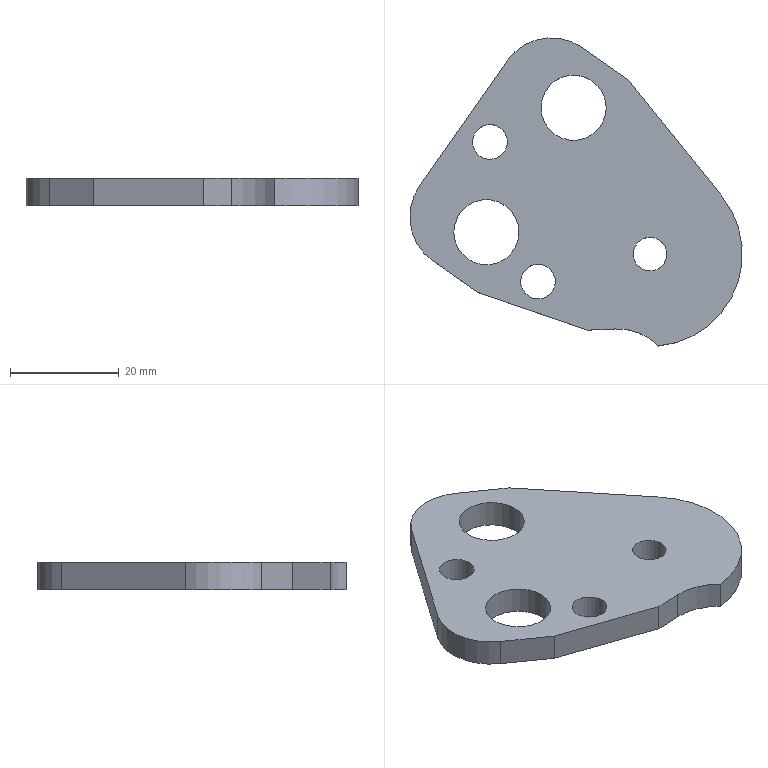Part | NX | features solid 2 | 1 solid | 17 faces | box 61.243 x 56.752 x 5 mm | volume 9744 mm3 | cylinder 9 | plane 8 | commonest cylinder face diameters 6.4 x2 12 x2 20 x2 6.2 x1 21 x1 34 x1
STEP:
#1=CARTESIAN_POINT('',(534.756,-127.127,79.));
#2=VERTEX_POINT('',#1);
#3=CARTESIAN_POINT('',(517.287,-105.544,79.));
#4=VERTEX_POINT('',#3);
#5=CARTESIAN_POINT('',(529.87,-121.089,79.));
#6=DIRECTION('',(-0.6291,0.7773,0.));
#7=VECTOR('',#6,1000.);
#8=LINE('',#5,#7);
#9=EDGE_CURVE('',#2,#4,#8,.T.);
#10=ORIENTED_EDGE('',*,*,#9,.F.);
#11=CARTESIAN_POINT('',(534.756,-127.127,74.));
#12=VERTEX_POINT('',#11);
#13=CARTESIAN_POINT('',(534.756,-127.127,74.));
#14=DIRECTION('',(0.,0.,1.));
#15=VECTOR('',#14,1000.);
#16=LINE('',#13,#15);
#17=EDGE_CURVE('',#12,#2,#16,.T.);
#18=ORIENTED_EDGE('',*,*,#17,.F.);
#19=CARTESIAN_POINT('',(517.287,-105.544,74.));
#20=VERTEX_POINT('',#19);
#21=CARTESIAN_POINT('',(529.87,-121.089,74.));
#22=DIRECTION('',(0.6291,-0.7773,0.));
#23=VECTOR('',#22,1000.);
#24=LINE('',#21,#23);
#25=EDGE_CURVE('',#20,#12,#24,.T.);
#26=ORIENTED_EDGE('',*,*,#25,.F.);
#27=CARTESIAN_POINT('',(517.287,-105.544,74.));
#28=DIRECTION('',(0.,0.,1.));
#29=VECTOR('',#28,1000.);
#30=LINE('',#27,#29);
#31=EDGE_CURVE('',#20,#4,#30,.T.);
#32=ORIENTED_EDGE('',*,*,#31,.T.);
#33=EDGE_LOOP('',(#10,#18,#26,#32));
#34=FACE_BOUND('',#33,.T.);
#35=CARTESIAN_POINT('',(529.87,-121.089,74.));
#36=DIRECTION('',(-0.7773,-0.6291,0.));
#37=DIRECTION('',(0.,0.,-1.));
#38=AXIS2_PLACEMENT_3D('',#35,#36,#37);
#39=PLANE('',#38);
#40=ADVANCED_FACE('',(#34),#39,.F.);
#41=CARTESIAN_POINT('',(515.152,-151.612,79.));
#42=VERTEX_POINT('',#41);
#43=CARTESIAN_POINT('',(510.031,-151.839,79.));
#44=VERTEX_POINT('',#43);
#45=CARTESIAN_POINT('',(515.285,-151.606,79.));
#46=DIRECTION('',(-0.999,-0.04437,0.));
#47=VECTOR('',#46,1000.);
#48=LINE('',#45,#47);
#49=EDGE_CURVE('',#42,#44,#48,.T.);
#50=ORIENTED_EDGE('',*,*,#49,.F.);
#51=CARTESIAN_POINT('',(523.093,-154.751,79.));
#52=VERTEX_POINT('',#51);
#53=CARTESIAN_POINT('',(515.596,-162.103,79.));
#54=DIRECTION('',(0.,0.,1.));
#55=DIRECTION('',(1.,0.,0.));
#56=AXIS2_PLACEMENT_3D('',#53,#54,#55);
#57=CIRCLE('',#56,10.5);
#58=EDGE_CURVE('',#52,#42,#57,.T.);
#59=ORIENTED_EDGE('',*,*,#58,.F.);
#60=CARTESIAN_POINT('',(521.542,-137.822,79.));
#61=DIRECTION('',(0.,0.,-1.));
#62=DIRECTION('',(0.5736,0.8192,0.));
#63=AXIS2_PLACEMENT_3D('',#60,#61,#62);
#64=CIRCLE('',#63,17.);
#65=EDGE_CURVE('',#2,#52,#64,.T.);
#66=ORIENTED_EDGE('',*,*,#65,.F.);
#67=ORIENTED_EDGE('',*,*,#9,.T.);
#68=CARTESIAN_POINT('',(509.095,-99.808,79.));
#69=VERTEX_POINT('',#68);
#70=CARTESIAN_POINT('',(528.218,-113.198,79.));
#71=DIRECTION('',(0.8192,-0.5736,0.));
#72=VECTOR('',#71,1000.);
#73=LINE('',#70,#72);
#74=EDGE_CURVE('',#69,#4,#73,.T.);
#75=ORIENTED_EDGE('',*,*,#74,.F.);
#76=CARTESIAN_POINT('',(495.168,-102.264,79.));
#77=VERTEX_POINT('',#76);
#78=CARTESIAN_POINT('',(503.359,-107.999,79.));
#79=DIRECTION('',(0.,0.,1.));
#80=DIRECTION('',(0.9397,0.342,0.));
#81=AXIS2_PLACEMENT_3D('',#78,#79,#80);
#82=CIRCLE('',#81,10.);
#83=EDGE_CURVE('',#69,#77,#82,.T.);
#84=ORIENTED_EDGE('',*,*,#83,.T.);
#85=CARTESIAN_POINT('',(479.108,-125.2,79.));
#86=VERTEX_POINT('',#85);
#87=CARTESIAN_POINT('',(487.138,-113.732,79.));
#88=DIRECTION('',(0.5736,0.8192,0.));
#89=VECTOR('',#88,1000.);
#90=LINE('',#87,#89);
#91=EDGE_CURVE('',#86,#77,#90,.T.);
#92=ORIENTED_EDGE('',*,*,#91,.F.);
#93=CARTESIAN_POINT('',(481.564,-139.127,79.));
#94=VERTEX_POINT('',#93);
#95=CARTESIAN_POINT('',(487.299,-130.936,79.));
#96=DIRECTION('',(0.,0.,1.));
#97=DIRECTION('',(0.9397,0.342,0.));
#98=AXIS2_PLACEMENT_3D('',#95,#96,#97);
#99=CIRCLE('',#98,10.);
#100=EDGE_CURVE('',#86,#94,#99,.T.);
#101=ORIENTED_EDGE('',*,*,#100,.T.);
#102=CARTESIAN_POINT('',(489.755,-144.863,79.));
#103=VERTEX_POINT('',#102);
#104=CARTESIAN_POINT('',(500.687,-152.517,79.));
#105=DIRECTION('',(-0.8192,0.5736,0.));
#106=VECTOR('',#105,1000.);
#107=LINE('',#104,#106);
#108=EDGE_CURVE('',#103,#94,#107,.T.);
#109=ORIENTED_EDGE('',*,*,#108,.F.);
#110=CARTESIAN_POINT('',(508.667,-151.37,79.));
#111=DIRECTION('',(0.9456,-0.3254,0.));
#112=VECTOR('',#111,1000.);
#113=LINE('',#110,#112);
#114=EDGE_CURVE('',#103,#44,#113,.T.);
#115=ORIENTED_EDGE('',*,*,#114,.T.);
#116=EDGE_LOOP('',(#50,#59,#66,#67,#75,#84,#92,#101,#109,#115));
#117=FACE_BOUND('',#116,.T.);
#118=CARTESIAN_POINT('',(493.888,-114.552,79.));
#119=VERTEX_POINT('',#118);
#120=CARTESIAN_POINT('',(492.053,-117.173,79.));
#121=DIRECTION('',(0.,0.,-1.));
#122=DIRECTION('',(0.5736,0.8192,0.));
#123=AXIS2_PLACEMENT_3D('',#120,#121,#122);
#124=CIRCLE('',#123,3.2);
#125=EDGE_CURVE('',#119,#119,#124,.T.);
#126=ORIENTED_EDGE('',*,*,#125,.T.);
#127=EDGE_LOOP('',(#126));
#128=FACE_BOUND('',#127,.T.);
#129=CARTESIAN_POINT('',(502.732,-140.277,79.));
#130=VERTEX_POINT('',#129);
#131=CARTESIAN_POINT('',(500.897,-142.898,79.));
#132=DIRECTION('',(0.,0.,-1.));
#133=DIRECTION('',(0.5736,0.8192,0.));
#134=AXIS2_PLACEMENT_3D('',#131,#132,#133);
#135=CIRCLE('',#134,3.2);
#136=EDGE_CURVE('',#130,#130,#135,.T.);
#137=ORIENTED_EDGE('',*,*,#136,.T.);
#138=EDGE_LOOP('',(#137));
#139=FACE_BOUND('',#138,.T.);
#140=CARTESIAN_POINT('',(494.837,-128.889,79.));
#141=VERTEX_POINT('',#140);
#142=CARTESIAN_POINT('',(491.395,-133.804,79.));
#143=DIRECTION('',(0.,0.,-1.));
#144=DIRECTION('',(0.5736,0.8192,0.));
#145=AXIS2_PLACEMENT_3D('',#142,#143,#144);
#146=CIRCLE('',#145,6.);
#147=EDGE_CURVE('',#141,#141,#146,.T.);
#148=ORIENTED_EDGE('',*,*,#147,.T.);
#149=EDGE_LOOP('',(#148));
#150=FACE_BOUND('',#149,.T.);
#151=CARTESIAN_POINT('',(510.897,-105.952,79.));
#152=VERTEX_POINT('',#151);
#153=CARTESIAN_POINT('',(507.455,-110.867,79.));
#154=DIRECTION('',(0.,0.,-1.));
#155=DIRECTION('',(0.5736,0.8192,0.));
#156=AXIS2_PLACEMENT_3D('',#153,#154,#155);
#157=CIRCLE('',#156,6.);
#158=EDGE_CURVE('',#152,#152,#157,.T.);
#159=ORIENTED_EDGE('',*,*,#158,.T.);
#160=EDGE_LOOP('',(#159));
#161=FACE_BOUND('',#160,.T.);
#162=CARTESIAN_POINT('',(523.32,-135.283,79.));
#163=VERTEX_POINT('',#162);
#164=CARTESIAN_POINT('',(521.542,-137.822,79.));
#165=DIRECTION('',(0.,0.,-1.));
#166=DIRECTION('',(0.5736,0.8192,0.));
#167=AXIS2_PLACEMENT_3D('',#164,#165,#166);
#168=CIRCLE('',#167,3.1);
#169=EDGE_CURVE('',#163,#163,#168,.T.);
#170=ORIENTED_EDGE('',*,*,#169,.T.);
#171=EDGE_LOOP('',(#170));
#172=FACE_BOUND('',#171,.T.);
#173=CARTESIAN_POINT('',(514.453,-132.858,79.));
#174=DIRECTION('',(0.,0.,1.));
#175=DIRECTION('',(-0.5736,-0.8192,0.));
#176=AXIS2_PLACEMENT_3D('',#173,#174,#175);
#177=PLANE('',#176);
#178=ADVANCED_FACE('',(#117,#128,#139,#150,#161,#172),#177,.T.);
#179=ORIENTED_EDGE('',*,*,#31,.F.);
#180=CARTESIAN_POINT('',(509.095,-99.808,74.));
#181=VERTEX_POINT('',#180);
#182=CARTESIAN_POINT('',(528.218,-113.198,74.));
#183=DIRECTION('',(-0.8192,0.5736,0.));
#184=VECTOR('',#183,1000.);
#185=LINE('',#182,#184);
#186=EDGE_CURVE('',#20,#181,#185,.T.);
#187=ORIENTED_EDGE('',*,*,#186,.T.);
#188=CARTESIAN_POINT('',(509.095,-99.808,74.));
#189=DIRECTION('',(0.,0.,1.));
#190=VECTOR('',#189,1000.);
#191=LINE('',#188,#190);
#192=EDGE_CURVE('',#181,#69,#191,.T.);
#193=ORIENTED_EDGE('',*,*,#192,.T.);
#194=ORIENTED_EDGE('',*,*,#74,.T.);
#195=EDGE_LOOP('',(#179,#187,#193,#194));
#196=FACE_BOUND('',#195,.T.);
#197=CARTESIAN_POINT('',(528.218,-113.198,74.));
#198=DIRECTION('',(0.5736,0.8192,0.));
#199=DIRECTION('',(0.,0.,1.));
#200=AXIS2_PLACEMENT_3D('',#197,#198,#199);
#201=PLANE('',#200);
#202=ADVANCED_FACE('',(#196),#201,.T.);
#203=CARTESIAN_POINT('',(510.031,-151.839,74.));
#204=VERTEX_POINT('',#203);
#205=CARTESIAN_POINT('',(515.152,-151.612,74.));
#206=VERTEX_POINT('',#205);
#207=CARTESIAN_POINT('',(515.285,-151.606,74.));
#208=DIRECTION('',(0.999,0.04437,0.));
#209=VECTOR('',#208,1000.);
#210=LINE('',#207,#209);
#211=EDGE_CURVE('',#204,#206,#210,.T.);
#212=ORIENTED_EDGE('',*,*,#211,.F.);
#213=CARTESIAN_POINT('',(489.755,-144.863,74.));
#214=VERTEX_POINT('',#213);
#215=CARTESIAN_POINT('',(508.667,-151.37,74.));
#216=DIRECTION('',(-0.9456,0.3254,0.));
#217=VECTOR('',#216,1000.);
#218=LINE('',#215,#217);
#219=EDGE_CURVE('',#204,#214,#218,.T.);
#220=ORIENTED_EDGE('',*,*,#219,.T.);
#221=CARTESIAN_POINT('',(481.564,-139.127,74.));
#222=VERTEX_POINT('',#221);
#223=CARTESIAN_POINT('',(500.687,-152.517,74.));
#224=DIRECTION('',(0.8192,-0.5736,0.));
#225=VECTOR('',#224,1000.);
#226=LINE('',#223,#225);
#227=EDGE_CURVE('',#222,#214,#226,.T.);
#228=ORIENTED_EDGE('',*,*,#227,.F.);
#229=CARTESIAN_POINT('',(479.108,-125.2,74.));
#230=VERTEX_POINT('',#229);
#231=CARTESIAN_POINT('',(487.299,-130.936,74.));
#232=DIRECTION('',(0.,0.,-1.));
#233=DIRECTION('',(-0.9397,-0.342,0.));
#234=AXIS2_PLACEMENT_3D('',#231,#232,#233);
#235=CIRCLE('',#234,10.);
#236=EDGE_CURVE('',#222,#230,#235,.T.);
#237=ORIENTED_EDGE('',*,*,#236,.T.);
#238=CARTESIAN_POINT('',(495.168,-102.264,74.));
#239=VERTEX_POINT('',#238);
#240=CARTESIAN_POINT('',(487.138,-113.732,74.));
#241=DIRECTION('',(-0.5736,-0.8192,0.));
#242=VECTOR('',#241,1000.);
#243=LINE('',#240,#242);
#244=EDGE_CURVE('',#239,#230,#243,.T.);
#245=ORIENTED_EDGE('',*,*,#244,.F.);
#246=CARTESIAN_POINT('',(503.359,-107.999,74.));
#247=DIRECTION('',(0.,0.,-1.));
#248=DIRECTION('',(-0.9397,-0.342,0.));
#249=AXIS2_PLACEMENT_3D('',#246,#247,#248);
#250=CIRCLE('',#249,10.);
#251=EDGE_CURVE('',#239,#181,#250,.T.);
#252=ORIENTED_EDGE('',*,*,#251,.T.);
#253=ORIENTED_EDGE('',*,*,#186,.F.);
#254=ORIENTED_EDGE('',*,*,#25,.T.);
#255=CARTESIAN_POINT('',(523.093,-154.751,74.));
#256=VERTEX_POINT('',#255);
#257=CARTESIAN_POINT('',(521.542,-137.822,74.));
#258=DIRECTION('',(0.,0.,1.));
#259=DIRECTION('',(-0.5736,-0.8192,0.));
#260=AXIS2_PLACEMENT_3D('',#257,#258,#259);
#261=CIRCLE('',#260,17.);
#262=EDGE_CURVE('',#256,#12,#261,.T.);
#263=ORIENTED_EDGE('',*,*,#262,.F.);
#264=CARTESIAN_POINT('',(515.596,-162.103,74.));
#265=DIRECTION('',(0.,0.,-1.));
#266=DIRECTION('',(-1.,0.,0.));
#267=AXIS2_PLACEMENT_3D('',#264,#265,#266);
#268=CIRCLE('',#267,10.5);
#269=EDGE_CURVE('',#206,#256,#268,.T.);
#270=ORIENTED_EDGE('',*,*,#269,.F.);
#271=EDGE_LOOP('',(#212,#220,#228,#237,#245,#252,#253,#254,#263,#270));
#272=FACE_BOUND('',#271,.T.);
#273=CARTESIAN_POINT('',(490.217,-119.795,74.));
#274=VERTEX_POINT('',#273);
#275=CARTESIAN_POINT('',(492.053,-117.173,74.));
#276=DIRECTION('',(0.,0.,1.));
#277=DIRECTION('',(-0.5736,-0.8192,0.));
#278=AXIS2_PLACEMENT_3D('',#275,#276,#277);
#279=CIRCLE('',#278,3.2);
#280=EDGE_CURVE('',#274,#274,#279,.T.);
#281=ORIENTED_EDGE('',*,*,#280,.T.);
#282=EDGE_LOOP('',(#281));
#283=FACE_BOUND('',#282,.T.);
#284=CARTESIAN_POINT('',(499.061,-145.52,74.));
#285=VERTEX_POINT('',#284);
#286=CARTESIAN_POINT('',(500.897,-142.898,74.));
#287=DIRECTION('',(0.,0.,1.));
#288=DIRECTION('',(-0.5736,-0.8192,0.));
#289=AXIS2_PLACEMENT_3D('',#286,#287,#288);
#290=CIRCLE('',#289,3.2);
#291=EDGE_CURVE('',#285,#285,#290,.T.);
#292=ORIENTED_EDGE('',*,*,#291,.T.);
#293=EDGE_LOOP('',(#292));
#294=FACE_BOUND('',#293,.T.);
#295=CARTESIAN_POINT('',(487.954,-138.719,74.));
#296=VERTEX_POINT('',#295);
#297=CARTESIAN_POINT('',(491.395,-133.804,74.));
#298=DIRECTION('',(0.,0.,1.));
#299=DIRECTION('',(-0.5736,-0.8192,0.));
#300=AXIS2_PLACEMENT_3D('',#297,#298,#299);
#301=CIRCLE('',#300,6.);
#302=EDGE_CURVE('',#296,#296,#301,.T.);
#303=ORIENTED_EDGE('',*,*,#302,.T.);
#304=EDGE_LOOP('',(#303));
#305=FACE_BOUND('',#304,.T.);
#306=CARTESIAN_POINT('',(504.014,-115.782,74.));
#307=VERTEX_POINT('',#306);
#308=CARTESIAN_POINT('',(507.455,-110.867,74.));
#309=DIRECTION('',(0.,0.,1.));
#310=DIRECTION('',(-0.5736,-0.8192,0.));
#311=AXIS2_PLACEMENT_3D('',#308,#309,#310);
#312=CIRCLE('',#311,6.);
#313=EDGE_CURVE('',#307,#307,#312,.T.);
#314=ORIENTED_EDGE('',*,*,#313,.T.);
#315=EDGE_LOOP('',(#314));
#316=FACE_BOUND('',#315,.T.);
#317=CARTESIAN_POINT('',(519.764,-140.361,74.));
#318=VERTEX_POINT('',#317);
#319=CARTESIAN_POINT('',(521.542,-137.822,74.));
#320=DIRECTION('',(0.,0.,1.));
#321=DIRECTION('',(-0.5736,-0.8192,0.));
#322=AXIS2_PLACEMENT_3D('',#319,#320,#321);
#323=CIRCLE('',#322,3.1);
#324=EDGE_CURVE('',#318,#318,#323,.T.);
#325=ORIENTED_EDGE('',*,*,#324,.T.);
#326=EDGE_LOOP('',(#325));
#327=FACE_BOUND('',#326,.T.);
#328=CARTESIAN_POINT('',(514.453,-132.858,74.));
#329=DIRECTION('',(0.,0.,-1.));
#330=DIRECTION('',(0.5736,0.8192,0.));
#331=AXIS2_PLACEMENT_3D('',#328,#329,#330);
#332=PLANE('',#331);
#333=ADVANCED_FACE('',(#272,#283,#294,#305,#316,#327),#332,.T.);
#334=CARTESIAN_POINT('',(489.755,-144.863,74.));
#335=DIRECTION('',(0.,0.,1.));
#336=VECTOR('',#335,1000.);
#337=LINE('',#334,#336);
#338=EDGE_CURVE('',#214,#103,#337,.T.);
#339=ORIENTED_EDGE('',*,*,#338,.T.);
#340=ORIENTED_EDGE('',*,*,#108,.T.);
#341=CARTESIAN_POINT('',(481.564,-139.127,74.));
#342=DIRECTION('',(0.,0.,1.));
#343=VECTOR('',#342,1000.);
#344=LINE('',#341,#343);
#345=EDGE_CURVE('',#94,#222,#344,.F.);
#346=ORIENTED_EDGE('',*,*,#345,.T.);
#347=ORIENTED_EDGE('',*,*,#227,.T.);
#348=EDGE_LOOP('',(#339,#340,#346,#347));
#349=FACE_BOUND('',#348,.T.);
#350=CARTESIAN_POINT('',(500.687,-152.517,74.));
#351=DIRECTION('',(-0.5736,-0.8192,0.));
#352=DIRECTION('',(0.,0.,-1.));
#353=AXIS2_PLACEMENT_3D('',#350,#351,#352);
#354=PLANE('',#353);
#355=ADVANCED_FACE('',(#349),#354,.T.);
#356=CARTESIAN_POINT('',(523.093,-154.751,250.));
#357=DIRECTION('',(0.,0.,1.));
#358=VECTOR('',#357,1000.);
#359=LINE('',#356,#358);
#360=EDGE_CURVE('',#256,#52,#359,.T.);
#361=ORIENTED_EDGE('',*,*,#360,.F.);
#362=ORIENTED_EDGE('',*,*,#262,.T.);
#363=ORIENTED_EDGE('',*,*,#17,.T.);
#364=ORIENTED_EDGE('',*,*,#65,.T.);
#365=EDGE_LOOP('',(#361,#362,#363,#364));
#366=FACE_BOUND('',#365,.T.);
#367=CARTESIAN_POINT('',(521.542,-137.822,74.));
#368=DIRECTION('',(0.,0.,1.));
#369=DIRECTION('',(-0.5736,-0.8192,0.));
#370=AXIS2_PLACEMENT_3D('',#367,#368,#369);
#371=CYLINDRICAL_SURFACE('',#370,17.);
#372=ADVANCED_FACE('',(#366),#371,.T.);
#373=ORIENTED_EDGE('',*,*,#244,.T.);
#374=CARTESIAN_POINT('',(479.108,-125.2,74.));
#375=DIRECTION('',(0.,0.,1.));
#376=VECTOR('',#375,1000.);
#377=LINE('',#374,#376);
#378=EDGE_CURVE('',#230,#86,#377,.T.);
#379=ORIENTED_EDGE('',*,*,#378,.T.);
#380=ORIENTED_EDGE('',*,*,#91,.T.);
#381=CARTESIAN_POINT('',(495.168,-102.264,74.));
#382=DIRECTION('',(0.,0.,1.));
#383=VECTOR('',#382,1000.);
#384=LINE('',#381,#383);
#385=EDGE_CURVE('',#77,#239,#384,.F.);
#386=ORIENTED_EDGE('',*,*,#385,.T.);
#387=EDGE_LOOP('',(#373,#379,#380,#386));
#388=FACE_BOUND('',#387,.T.);
#389=CARTESIAN_POINT('',(487.138,-113.732,74.));
#390=DIRECTION('',(-0.8192,0.5736,0.));
#391=DIRECTION('',(0.,0.,-1.));
#392=AXIS2_PLACEMENT_3D('',#389,#390,#391);
#393=PLANE('',#392);
#394=ADVANCED_FACE('',(#388),#393,.T.);
#395=ORIENTED_EDGE('',*,*,#169,.F.);
#396=EDGE_LOOP('',(#395));
#397=FACE_BOUND('',#396,.T.);
#398=ORIENTED_EDGE('',*,*,#324,.F.);
#399=EDGE_LOOP('',(#398));
#400=FACE_BOUND('',#399,.T.);
#401=CARTESIAN_POINT('',(521.542,-137.822,74.));
#402=DIRECTION('',(0.,0.,1.));
#403=DIRECTION('',(-0.5736,-0.8192,0.));
#404=AXIS2_PLACEMENT_3D('',#401,#402,#403);
#405=CYLINDRICAL_SURFACE('',#404,3.1);
#406=ADVANCED_FACE('',(#397,#400),#405,.F.);
#407=ORIENTED_EDGE('',*,*,#158,.F.);
#408=EDGE_LOOP('',(#407));
#409=FACE_BOUND('',#408,.T.);
#410=ORIENTED_EDGE('',*,*,#313,.F.);
#411=EDGE_LOOP('',(#410));
#412=FACE_BOUND('',#411,.T.);
#413=CARTESIAN_POINT('',(507.455,-110.867,74.));
#414=DIRECTION('',(0.,0.,1.));
#415=DIRECTION('',(-0.5736,-0.8192,0.));
#416=AXIS2_PLACEMENT_3D('',#413,#414,#415);
#417=CYLINDRICAL_SURFACE('',#416,6.);
#418=ADVANCED_FACE('',(#409,#412),#417,.F.);
#419=ORIENTED_EDGE('',*,*,#147,.F.);
#420=EDGE_LOOP('',(#419));
#421=FACE_BOUND('',#420,.T.);
#422=ORIENTED_EDGE('',*,*,#302,.F.);
#423=EDGE_LOOP('',(#422));
#424=FACE_BOUND('',#423,.T.);
#425=CARTESIAN_POINT('',(491.395,-133.804,74.));
#426=DIRECTION('',(0.,0.,1.));
#427=DIRECTION('',(-0.5736,-0.8192,0.));
#428=AXIS2_PLACEMENT_3D('',#425,#426,#427);
#429=CYLINDRICAL_SURFACE('',#428,6.);
#430=ADVANCED_FACE('',(#421,#424),#429,.F.);
#431=ORIENTED_EDGE('',*,*,#136,.F.);
#432=EDGE_LOOP('',(#431));
#433=FACE_BOUND('',#432,.T.);
#434=ORIENTED_EDGE('',*,*,#291,.F.);
#435=EDGE_LOOP('',(#434));
#436=FACE_BOUND('',#435,.T.);
#437=CARTESIAN_POINT('',(500.897,-142.898,74.));
#438=DIRECTION('',(0.,0.,1.));
#439=DIRECTION('',(-0.5736,-0.8192,0.));
#440=AXIS2_PLACEMENT_3D('',#437,#438,#439);
#441=CYLINDRICAL_SURFACE('',#440,3.2);
#442=ADVANCED_FACE('',(#433,#436),#441,.F.);
#443=ORIENTED_EDGE('',*,*,#125,.F.);
#444=EDGE_LOOP('',(#443));
#445=FACE_BOUND('',#444,.T.);
#446=ORIENTED_EDGE('',*,*,#280,.F.);
#447=EDGE_LOOP('',(#446));
#448=FACE_BOUND('',#447,.T.);
#449=CARTESIAN_POINT('',(492.053,-117.173,74.));
#450=DIRECTION('',(0.,0.,1.));
#451=DIRECTION('',(-0.5736,-0.8192,0.));
#452=AXIS2_PLACEMENT_3D('',#449,#450,#451);
#453=CYLINDRICAL_SURFACE('',#452,3.2);
#454=ADVANCED_FACE('',(#445,#448),#453,.F.);
#455=ORIENTED_EDGE('',*,*,#236,.F.);
#456=ORIENTED_EDGE('',*,*,#345,.F.);
#457=ORIENTED_EDGE('',*,*,#100,.F.);
#458=ORIENTED_EDGE('',*,*,#378,.F.);
#459=EDGE_LOOP('',(#455,#456,#457,#458));
#460=FACE_BOUND('',#459,.T.);
#461=CARTESIAN_POINT('',(487.299,-130.936,74.));
#462=DIRECTION('',(0.,0.,1.));
#463=DIRECTION('',(0.9397,0.342,0.));
#464=AXIS2_PLACEMENT_3D('',#461,#462,#463);
#465=CYLINDRICAL_SURFACE('',#464,10.);
#466=ADVANCED_FACE('',(#460),#465,.T.);
#467=ORIENTED_EDGE('',*,*,#251,.F.);
#468=ORIENTED_EDGE('',*,*,#385,.F.);
#469=ORIENTED_EDGE('',*,*,#83,.F.);
#470=ORIENTED_EDGE('',*,*,#192,.F.);
#471=EDGE_LOOP('',(#467,#468,#469,#470));
#472=FACE_BOUND('',#471,.T.);
#473=CARTESIAN_POINT('',(503.359,-107.999,74.));
#474=DIRECTION('',(0.,0.,1.));
#475=DIRECTION('',(0.9397,0.342,0.));
#476=AXIS2_PLACEMENT_3D('',#473,#474,#475);
#477=CYLINDRICAL_SURFACE('',#476,10.);
#478=ADVANCED_FACE('',(#472),#477,.T.);
#479=ORIENTED_EDGE('',*,*,#219,.F.);
#480=CARTESIAN_POINT('',(510.031,-151.839,74.));
#481=DIRECTION('',(0.,0.,1.));
#482=VECTOR('',#481,1000.);
#483=LINE('',#480,#482);
#484=EDGE_CURVE('',#204,#44,#483,.T.);
#485=ORIENTED_EDGE('',*,*,#484,.T.);
#486=ORIENTED_EDGE('',*,*,#114,.F.);
#487=ORIENTED_EDGE('',*,*,#338,.F.);
#488=EDGE_LOOP('',(#479,#485,#486,#487));
#489=FACE_BOUND('',#488,.T.);
#490=CARTESIAN_POINT('',(508.667,-151.37,74.));
#491=DIRECTION('',(0.3254,0.9456,0.));
#492=DIRECTION('',(0.,0.,1.));
#493=AXIS2_PLACEMENT_3D('',#490,#491,#492);
#494=PLANE('',#493);
#495=ADVANCED_FACE('',(#489),#494,.F.);
#496=ORIENTED_EDGE('',*,*,#360,.T.);
#497=ORIENTED_EDGE('',*,*,#58,.T.);
#498=CARTESIAN_POINT('',(515.152,-151.612,0.));
#499=DIRECTION('',(0.,0.,1.));
#500=VECTOR('',#499,1000.);
#501=LINE('',#498,#500);
#502=EDGE_CURVE('',#206,#42,#501,.T.);
#503=ORIENTED_EDGE('',*,*,#502,.F.);
#504=ORIENTED_EDGE('',*,*,#269,.T.);
#505=EDGE_LOOP('',(#496,#497,#503,#504));
#506=FACE_BOUND('',#505,.T.);
#507=CARTESIAN_POINT('',(515.596,-162.103,0.));
#508=DIRECTION('',(0.,0.,1.));
#509=DIRECTION('',(1.,0.,0.));
#510=AXIS2_PLACEMENT_3D('',#507,#508,#509);
#511=CYLINDRICAL_SURFACE('',#510,10.5);
#512=ADVANCED_FACE('',(#506),#511,.F.);
#513=ORIENTED_EDGE('',*,*,#502,.T.);
#514=ORIENTED_EDGE('',*,*,#49,.T.);
#515=ORIENTED_EDGE('',*,*,#484,.F.);
#516=ORIENTED_EDGE('',*,*,#211,.T.);
#517=EDGE_LOOP('',(#513,#514,#515,#516));
#518=FACE_BOUND('',#517,.T.);
#519=CARTESIAN_POINT('',(515.152,-151.612,0.));
#520=DIRECTION('',(-0.04437,0.999,0.));
#521=DIRECTION('',(-0.999,-0.04437,0.));
#522=AXIS2_PLACEMENT_3D('',#519,#520,#521);
#523=PLANE('',#522);
#524=ADVANCED_FACE('',(#518),#523,.F.);
#525=CLOSED_SHELL('',(#40,#178,#202,#333,#355,#372,#394,#406,#418,#430,#442,#454,#466,#478,#495,#512,#524));
#526=MANIFOLD_SOLID_BREP('',#525);
#527=(LENGTH_UNIT()NAMED_UNIT(*)SI_UNIT(.MILLI.,.METRE.));
#528=UNCERTAINTY_MEASURE_WITH_UNIT(LENGTH_MEASURE(0.00001),#527,'','');
#529=(NAMED_UNIT(*)PLANE_ANGLE_UNIT()SI_UNIT($,.RADIAN.));
#530=(NAMED_UNIT(*)SI_UNIT($,.STERADIAN.)SOLID_ANGLE_UNIT());
#531=(GEOMETRIC_REPRESENTATION_CONTEXT(3)GLOBAL_UNCERTAINTY_ASSIGNED_CONTEXT((#528))GLOBAL_UNIT_ASSIGNED_CONTEXT((#527,#529,#530))REPRESENTATION_CONTEXT('',''));
#532=ADVANCED_BREP_SHAPE_REPRESENTATION('',(#526),#531);